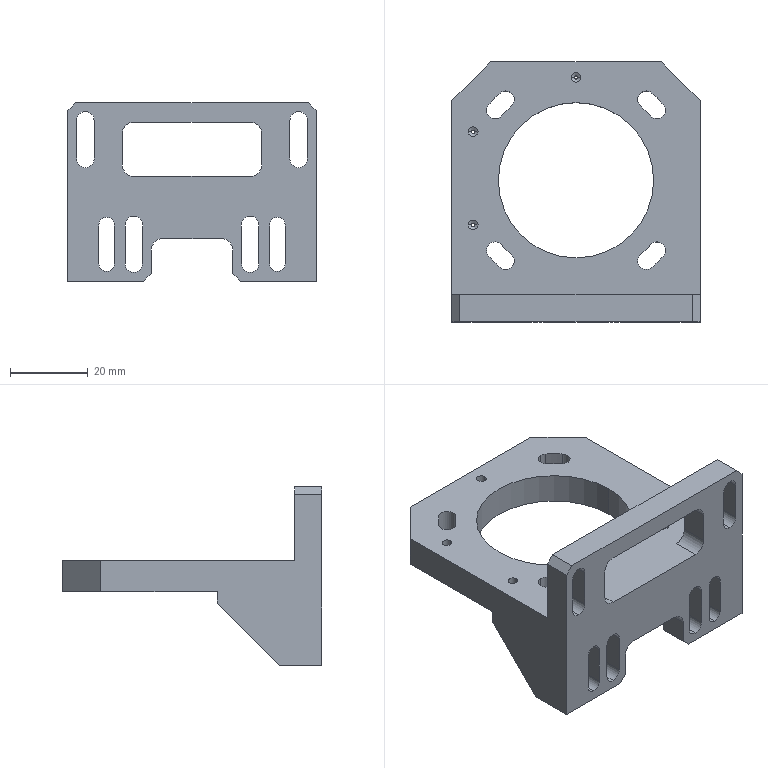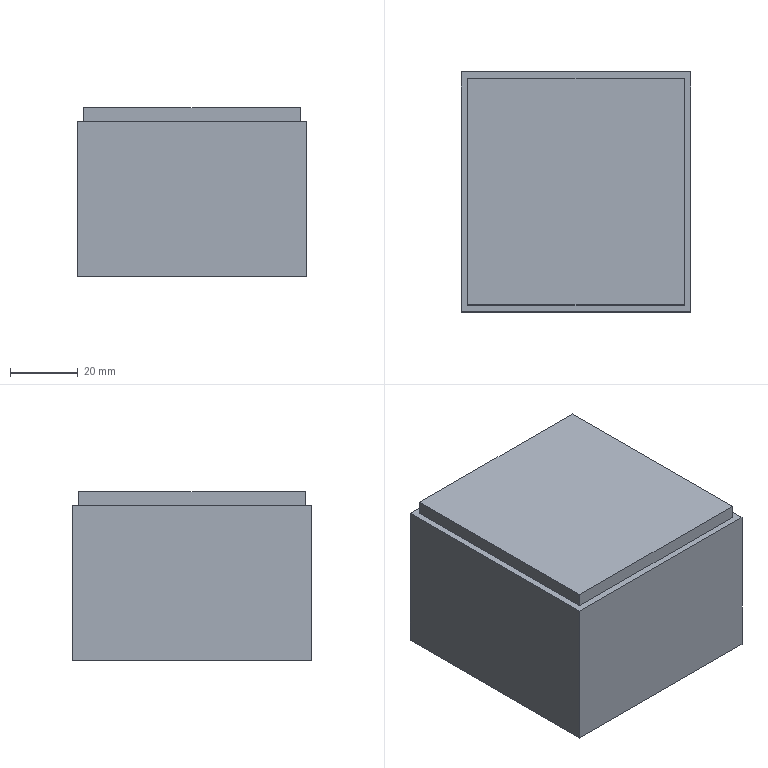CAM job | NX | 3+2 milling, drilling | part box 64 x 67 x 46 mm | stock box 68 x 71 x 50 mm
Tools:
number,name,description,diameter,corner_radius,flute_length,length,flutes
10,D10C,Milling Tool-5 Parameters,10.0,0.0,50.0,75.0,2
1,ZXZ,Milling Tool-5 Parameters,6.0,0.0,50.0,75.0,2
12,2.5ZT,Drilling Tool,2.5,0.0,35.0,50.0,2
6,D6JING,Milling Tool-5 Parameters,6.0,0.0,50.0,75.0,2
11,D10JING,Milling Tool-5 Parameters,10.0,0.0,50.0,75.0,2
5,D6R0.5,Milling Tool-5 Parameters,6.0,0.5,50.0,75.0,2
3,D3,Milling Tool-5 Parameters,3.0,0.0,50.0,75.0,2
7,D6A45,Milling Tool-5 Parameters,6.0,0.0,50.0,75.0,2
2,D63,Milling Tool-5 Parameters,63.0,0.0,50.0,75.0,2
Operations:
program,operation,operation_type,tool,method,geometry_group,spindle_rpm,surface_speed,feed_per_tooth,feed_cut,feed_plunge,cut_length_mm,path_length_mm,cut_time_min,machine_time_min
1,ZLEVEL_PROFILE,ZLevelMilling,D10C,METHOD,A,2500.0,78.0,0.5,2500.0,1000.0,129909.319,130012.319,51.982,51.992
1,FLOOR_WALL_1,VolumeBased25DMillingOperation,D10C,METHOD,A,2500.0,78.0,0.5,2500.0,1000.0,125535.725,131513.33,51.167,51.764
1,HOLE_MILLING,CylinderMilling,D10C,METHOD,A,2500.0,78.0,0.44,2200.0,100.0,16196.192,16318.692,7.362,7.374
1,DRILLING,Operation,ZXZ,METHOD,A,3500.0,65.0,0.0357,250.0,0.0,16.0,218.899,0.064,0.0843
1,DRILLING_COPY,Operation,2.5ZT,METHOD,A,2000.0,15.0,0.03,120.0,0.0,33.753,225.814,0.2813,0.3005
1,ZLEVEL_PROFILE_COPY,ZLevelMilling,D10JING,METHOD,A,5000.0,157.0,0.12,1200.0,1000.0,103.097,214.097,0.0867,0.0978
1,FLOOR_WALL_2,VolumeBased25DMillingOperation,D10JING,METHOD,A,7000.0,131.0,0.0893,1250.0,100.0,1007.008,1107.708,0.8056,0.8157
1,ZLEVEL_PROFILE_COPY_1,ZLevelMilling,D3,METHOD,A,5500.0,51.0,0.1136,1250.0,1000.0,7822.896,8355.662,6.271,6.325
1,ZLEVEL_PROFILE_COPY_2_COPY_COPY,ZLevelMilling,D6R0.5,METHOD,A,7000.0,131.0,0.2143,3000.0,1000.0,571.683,762.819,0.1939,0.2131
1,PLANAR_MILL_COPY,PlanarMilling,D6A45,METHOD,A,7500.0,141.0,0.0833,1250.0,100.0,152.749,211.749,0.1222,0.1281
1,PLANAR_MILL_COPY_COPY,PlanarMilling,D6A45,METHOD,A,7500.0,141.0,0.0833,1250.0,100.0,422.17,1498.299,0.3377,0.4453
2,FLOOR_WALL_COPY,VolumeBased25DMillingOperation,D63,METHOD,B,2000.0,395.0,0.3125,1250.0,100.0,17347.082,24817.593,13.878,14.625
2,FLOOR_WALL_COPY_COPY,VolumeBased25DMillingOperation,D10JING,METHOD,B,5000.0,157.0,0.125,1250.0,100.0,1076.997,1130.997,0.8616,0.867
2,FLOOR_WALL_1_1,VolumeBased25DMillingOperation,D10C,METHOD,B,2500.0,78.0,0.5,2500.0,1000.0,114744.633,119888.375,46.85,47.365
2,CAVITY_MILL,CavityMilling,D10C,METHOD,B,2500.0,78.0,0.44,2200.0,1000.0,24188.931,27230.846,13.09,13.395
2,ZLEVEL_PROFILE_COPY_2,ZLevelMilling,D6JING,METHOD,B,5000.0,94.0,0.15,1500.0,1000.0,2933.044,4227.209,2.166,2.295
2,FLOOR_WALL_2_1,VolumeBased25DMillingOperation,D6JING,METHOD,B,7000.0,131.0,0.0893,1250.0,100.0,1516.877,1892.541,1.214,1.251
2,ZLEVEL_PROFILE_COPY_2_COPY_COPY_COPY,ZLevelMilling,D6R0.5,METHOD,B,7000.0,131.0,0.2143,3000.0,1000.0,2205.889,2360.115,0.7387,0.7541
2,ZLEVEL_PROFILE_COPY_2_COPY_COPY_COPY_COPY,ZLevelMilling,D6R0.5,METHOD,B,7000.0,131.0,0.2143,3000.0,1000.0,2378.568,2596.244,0.7962,0.818
2,PLANAR_MILL_COPY_COPY_1,PlanarMilling,D6A45,METHOD,B,7500.0,141.0,0.0833,1250.0,100.0,212.923,397.723,0.1703,0.1888
2,PLANAR_MILL_COPY_COPY_1_COPY,PlanarMilling,D6A45,METHOD,B,7500.0,141.0,0.0833,1250.0,100.0,352.115,1099.233,0.2817,0.3564
3,ZLEVEL_PROFILE_COPY_3,ZLevelMilling,D10C,METHOD,C,2500.0,78.0,0.5,2500.0,1000.0,4182.16,4246.16,1.691,1.698
3,ZLEVEL_PROFILE_COPY_2_COPY,ZLevelMilling,D6JING,METHOD,C,5000.0,94.0,0.15,1500.0,1000.0,2175.04,3294.76,1.606,1.718
3,ZLEVEL_PROFILE_COPY_COPY,ZLevelMilling,D6JING,METHOD,C,5000.0,157.0,0.12,1200.0,1000.0,82.926,153.926,0.0697,0.0768
3,ZLEVEL_PROFILE_COPY_1_COPY,ZLevelMilling,D3,METHOD,C,5500.0,51.0,0.1136,1250.0,1000.0,20174.488,20674.732,16.159,16.209
3,ZLEVEL_PROFILE_COPY_1_COPY_COPY,ZLevelMilling,D3,METHOD,C,7500.0,70.0,0.0667,1000.0,1000.0,113.457,500.472,0.1135,0.1522
3,PLANAR_MILL_COPY_COPY_COPY_1,PlanarMilling,D6A45,METHOD,C,7500.0,141.0,0.0833,1250.0,100.0,307.187,837.189,0.2457,0.2987
3,刀补,ZLevelMilling,D3,METHOD,C,7500.0,70.0,0.0667,1000.0,1000.0,64.683,238.911,0.0647,0.0821